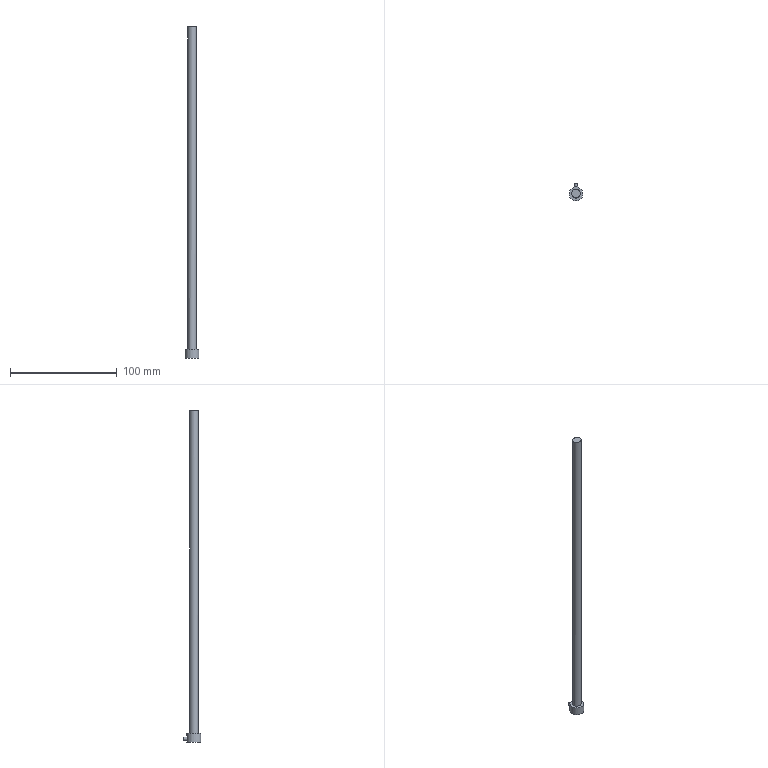Part | STEP file | E108-11-315 | 1 solid | 8 faces | box 13 x 16.5 x 310.586 mm | volume 16274 mm3 | cylinder 3 | plane 3 | spline 1 | cone 1 | commonest cylinder face diameters 3 x1 8 x1 13 x1
STEP:
#1=CARTESIAN_POINT('',(0.,0.,0.));
#2=DIRECTION('',(0.,0.,1.));
#3=DIRECTION('',(1.,0.,0.));
#4=AXIS2_PLACEMENT_3D('',#1,#2,#3);
#5=CARTESIAN_POINT('',(-3.864,1.032,309.65));
#6=VERTEX_POINT('',#5);
#7=CARTESIAN_POINT('',(-3.864,1.032,309.65));
#8=CARTESIAN_POINT('',(-3.979,0.6025,309.652));
#9=CARTESIAN_POINT('',(-4.022,0.147,309.665));
#10=CARTESIAN_POINT('',(-3.989,-0.2963,309.686));
#11=CARTESIAN_POINT('',(-3.956,-0.7395,309.708));
#12=CARTESIAN_POINT('',(-3.847,-1.183,309.739));
#13=CARTESIAN_POINT('',(-3.671,-1.589,309.777));
#14=CARTESIAN_POINT('',(-3.494,-1.998,309.816));
#15=CARTESIAN_POINT('',(-3.245,-2.381,309.862));
#16=CARTESIAN_POINT('',(-2.944,-2.708,309.911));
#17=CARTESIAN_POINT('',(-2.641,-3.038,309.961));
#18=CARTESIAN_POINT('',(-2.277,-3.319,310.016));
#19=CARTESIAN_POINT('',(-1.882,-3.53,310.071));
#20=CARTESIAN_POINT('',(-1.484,-3.742,310.126));
#21=CARTESIAN_POINT('',(-1.045,-3.887,310.183));
#22=CARTESIAN_POINT('',(-0.5993,-3.955,310.236));
#23=CARTESIAN_POINT('',(-0.1533,-4.022,310.289));
#24=CARTESIAN_POINT('',(0.3111,-4.013,310.339));
#25=CARTESIAN_POINT('',(0.7551,-3.928,310.383));
#26=CARTESIAN_POINT('',(1.197,-3.843,310.427));
#27=CARTESIAN_POINT('',(1.631,-3.68,310.466));
#28=CARTESIAN_POINT('',(2.021,-3.452,310.496));
#29=CARTESIAN_POINT('',(2.407,-3.226,310.527));
#30=CARTESIAN_POINT('',(2.761,-2.929,310.55));
#31=CARTESIAN_POINT('',(3.051,-2.586,310.565));
#32=CARTESIAN_POINT('',(3.34,-2.246,310.58));
#33=CARTESIAN_POINT('',(3.574,-1.851,310.587));
#34=CARTESIAN_POINT('',(3.734,-1.434,310.585));
#35=CARTESIAN_POINT('',(3.894,-1.018,310.584));
#36=CARTESIAN_POINT('',(3.984,-0.5693,310.575));
#37=CARTESIAN_POINT('',(3.998,-0.1245,310.559));
#38=CARTESIAN_POINT('',(4.012,0.3207,310.543));
#39=CARTESIAN_POINT('',(3.95,0.774,310.52));
#40=CARTESIAN_POINT('',(3.816,1.198,310.491));
#41=CARTESIAN_POINT('',(3.683,1.624,310.462));
#42=CARTESIAN_POINT('',(3.474,2.032,310.426));
#43=CARTESIAN_POINT('',(3.208,2.389,310.387));
#44=CARTESIAN_POINT('',(2.941,2.748,310.347));
#45=CARTESIAN_POINT('',(2.608,3.065,310.302));
#46=CARTESIAN_POINT('',(2.238,3.315,310.255));
#47=CARTESIAN_POINT('',(1.866,3.567,310.208));
#48=CARTESIAN_POINT('',(1.445,3.757,310.157));
#49=CARTESIAN_POINT('',(1.011,3.87,310.107));
#50=CARTESIAN_POINT('',(0.5759,3.984,310.056));
#51=CARTESIAN_POINT('',(0.1147,4.024,310.004));
#52=CARTESIAN_POINT('',(-0.3341,3.986,309.956));
#53=CARTESIAN_POINT('',(-0.7831,3.948,309.907));
#54=CARTESIAN_POINT('',(-1.232,3.832,309.86));
#55=CARTESIAN_POINT('',(-1.644,3.647,309.819));
#56=CARTESIAN_POINT('',(-2.054,3.462,309.778));
#57=CARTESIAN_POINT('',(-2.438,3.203,309.742));
#58=CARTESIAN_POINT('',(-2.764,2.891,309.714));
#59=CARTESIAN_POINT('',(-3.088,2.582,309.687));
#60=CARTESIAN_POINT('',(-3.363,2.212,309.667));
#61=CARTESIAN_POINT('',(-3.566,1.812,309.657));
#62=CARTESIAN_POINT('',(-3.692,1.564,309.651));
#63=CARTESIAN_POINT('',(-3.793,1.301,309.649));
#64=CARTESIAN_POINT('',(-3.864,1.032,309.65));
#65=B_SPLINE_CURVE_WITH_KNOTS('',3,(#7,#8,#9,#10,#11,#12,#13,#14,#15,#16,#17,#18,#19,#20,#21,#22,#23,#24,#25,#26,#27,#28,#29,#30,#31,#32,#33,#34,#35,#36,#37,#38,#39,#40,#41,#42,#43,#44,#45,#46,#47,#48,#49,#50,#51,#52,#53,#54,#55,#56,#57,#58,#59,#60,#61,#62,#63,#64),.UNSPECIFIED.,.T.,.F.,(1,3,3,3,3,3,3,3,3,3,3,3,3,3,3,3,3,3,3,3,3,1),(-0.03296,0.,0.0532,0.1064,0.1598,0.2137,0.2679,0.3222,0.3763,0.43,0.4834,0.5367,0.5899,0.6434,0.6971,0.751,0.8052,0.8594,0.9134,0.967,1.,1.053),.UNSPECIFIED.);
#66=CARTESIAN_POINT('',(0.,0.,108.));
#67=DIRECTION('',(0.,0.,-1.));
#68=DIRECTION('',(-1.,0.,0.));
#69=AXIS2_PLACEMENT_3D('',#66,#67,#68);
#70=CYLINDRICAL_SURFACE('',#69,4.);
#71=CARTESIAN_POINT('',(6.544,-201.65));
#72=CARTESIAN_POINT('',(6.521,-201.651));
#73=CARTESIAN_POINT('',(6.473,-201.653));
#74=CARTESIAN_POINT('',(6.401,-201.658));
#75=CARTESIAN_POINT('',(6.329,-201.666));
#76=CARTESIAN_POINT('',(6.258,-201.677));
#77=CARTESIAN_POINT('',(6.186,-201.69));
#78=CARTESIAN_POINT('',(6.115,-201.706));
#79=CARTESIAN_POINT('',(6.043,-201.725));
#80=CARTESIAN_POINT('',(5.972,-201.745));
#81=CARTESIAN_POINT('',(5.9,-201.768));
#82=CARTESIAN_POINT('',(5.829,-201.793));
#83=CARTESIAN_POINT('',(5.758,-201.82));
#84=CARTESIAN_POINT('',(5.686,-201.848));
#85=CARTESIAN_POINT('',(5.615,-201.878));
#86=CARTESIAN_POINT('',(5.544,-201.909));
#87=CARTESIAN_POINT('',(5.473,-201.941));
#88=CARTESIAN_POINT('',(5.402,-201.975));
#89=CARTESIAN_POINT('',(5.33,-202.009));
#90=CARTESIAN_POINT('',(5.259,-202.043));
#91=CARTESIAN_POINT('',(5.188,-202.078));
#92=CARTESIAN_POINT('',(5.117,-202.113));
#93=CARTESIAN_POINT('',(5.046,-202.148));
#94=CARTESIAN_POINT('',(4.975,-202.182));
#95=CARTESIAN_POINT('',(4.904,-202.217));
#96=CARTESIAN_POINT('',(4.833,-202.25));
#97=CARTESIAN_POINT('',(4.762,-202.282));
#98=CARTESIAN_POINT('',(4.69,-202.314));
#99=CARTESIAN_POINT('',(4.619,-202.344));
#100=CARTESIAN_POINT('',(4.548,-202.373));
#101=CARTESIAN_POINT('',(4.477,-202.401));
#102=CARTESIAN_POINT('',(4.405,-202.427));
#103=CARTESIAN_POINT('',(4.334,-202.451));
#104=CARTESIAN_POINT('',(4.262,-202.474));
#105=CARTESIAN_POINT('',(4.191,-202.494));
#106=CARTESIAN_POINT('',(4.12,-202.513));
#107=CARTESIAN_POINT('',(4.048,-202.53));
#108=CARTESIAN_POINT('',(3.976,-202.544));
#109=CARTESIAN_POINT('',(3.905,-202.557));
#110=CARTESIAN_POINT('',(3.834,-202.567));
#111=CARTESIAN_POINT('',(3.762,-202.575));
#112=CARTESIAN_POINT('',(3.69,-202.581));
#113=CARTESIAN_POINT('',(3.618,-202.584));
#114=CARTESIAN_POINT('',(3.547,-202.586));
#115=CARTESIAN_POINT('',(3.476,-202.585));
#116=CARTESIAN_POINT('',(3.404,-202.583));
#117=CARTESIAN_POINT('',(3.332,-202.578));
#118=CARTESIAN_POINT('',(3.26,-202.571));
#119=CARTESIAN_POINT('',(3.189,-202.562));
#120=CARTESIAN_POINT('',(3.117,-202.551));
#121=CARTESIAN_POINT('',(3.046,-202.538));
#122=CARTESIAN_POINT('',(2.974,-202.524));
#123=CARTESIAN_POINT('',(2.902,-202.508));
#124=CARTESIAN_POINT('',(2.831,-202.49));
#125=CARTESIAN_POINT('',(2.76,-202.47));
#126=CARTESIAN_POINT('',(2.688,-202.449));
#127=CARTESIAN_POINT('',(2.617,-202.426));
#128=CARTESIAN_POINT('',(2.545,-202.402));
#129=CARTESIAN_POINT('',(2.474,-202.377));
#130=CARTESIAN_POINT('',(2.403,-202.351));
#131=CARTESIAN_POINT('',(2.331,-202.323));
#132=CARTESIAN_POINT('',(2.26,-202.295));
#133=CARTESIAN_POINT('',(2.189,-202.265));
#134=CARTESIAN_POINT('',(2.118,-202.235));
#135=CARTESIAN_POINT('',(2.047,-202.205));
#136=CARTESIAN_POINT('',(1.975,-202.173));
#137=CARTESIAN_POINT('',(1.904,-202.142));
#138=CARTESIAN_POINT('',(1.833,-202.11));
#139=CARTESIAN_POINT('',(1.762,-202.078));
#140=CARTESIAN_POINT('',(1.691,-202.046));
#141=CARTESIAN_POINT('',(1.619,-202.014));
#142=CARTESIAN_POINT('',(1.548,-201.982));
#143=CARTESIAN_POINT('',(1.477,-201.951));
#144=CARTESIAN_POINT('',(1.406,-201.921));
#145=CARTESIAN_POINT('',(1.335,-201.891));
#146=CARTESIAN_POINT('',(1.263,-201.863));
#147=CARTESIAN_POINT('',(1.192,-201.835));
#148=CARTESIAN_POINT('',(1.121,-201.809));
#149=CARTESIAN_POINT('',(1.049,-201.784));
#150=CARTESIAN_POINT('',(0.9778,-201.761));
#151=CARTESIAN_POINT('',(0.9062,-201.74));
#152=CARTESIAN_POINT('',(0.8348,-201.721));
#153=CARTESIAN_POINT('',(0.7637,-201.704));
#154=CARTESIAN_POINT('',(0.6921,-201.688));
#155=CARTESIAN_POINT('',(0.6203,-201.676));
#156=CARTESIAN_POINT('',(0.5485,-201.665));
#157=CARTESIAN_POINT('',(0.4773,-201.657));
#158=CARTESIAN_POINT('',(0.4052,-201.652));
#159=CARTESIAN_POINT('',(0.3331,-201.65));
#160=CARTESIAN_POINT('',(0.285,-201.65));
#161=CARTESIAN_POINT('',(0.2611,-201.65));
#162=B_SPLINE_CURVE_WITH_KNOTS('',3,(#71,#72,#73,#74,#75,#76,#77,#78,#79,#80,#81,#82,#83,#84,#85,#86,#87,#88,#89,#90,#91,#92,#93,#94,#95,#96,#97,#98,#99,#100,#101,#102,#103,#104,#105,#106,#107,#108,#109,#110,#111,#112,#113,#114,#115,#116,#117,#118,#119,#120,#121,#122,#123,#124,#125,#126,#127,#128,#129,#130,#131,#132,#133,#134,#135,#136,#137,#138,#139,#140,#141,#142,#143,#144,#145,#146,#147,#148,#149,#150,#151,#152,#153,#154,#155,#156,#157,#158,#159,#160,#161),.UNSPECIFIED.,.F.,.F.,(4,1,1,1,1,1,1,1,1,1,1,1,1,1,1,1,1,1,1,1,1,1,1,1,1,1,1,1,1,1,1,1,1,1,1,1,1,1,1,1,1,1,1,1,1,1,1,1,1,1,1,1,1,1,1,1,1,1,1,1,1,1,1,1,1,1,1,1,1,1,1,1,1,1,1,1,1,1,1,1,1,1,1,1,1,1,1,1,4),(0.,0.01136,0.02273,0.03409,0.04545,0.05682,0.06818,0.07955,0.09091,0.1023,0.1136,0.125,0.1364,0.1477,0.1591,0.1705,0.1818,0.1932,0.2045,0.2159,0.2273,0.2386,0.25,0.2614,0.2727,0.2841,0.2955,0.3068,0.3182,0.3295,0.3409,0.3523,0.3636,0.375,0.3864,0.3977,0.4091,0.4205,0.4318,0.4432,0.4545,0.4659,0.4773,0.4886,0.5,0.5114,0.5227,0.5341,0.5455,0.5568,0.5682,0.5795,0.5909,0.6023,0.6136,0.625,0.6364,0.6477,0.6591,0.6705,0.6818,0.6932,0.7045,0.7159,0.7273,0.7386,0.75,0.7614,0.7727,0.7841,0.7955,0.8068,0.8182,0.8295,0.8409,0.8523,0.8636,0.875,0.8864,0.8977,0.9091,0.9205,0.9318,0.9432,0.9545,0.9659,0.9773,0.9886,1.),.QUASI_UNIFORM_KNOTS.);
#163=(GEOMETRIC_REPRESENTATION_CONTEXT(2)PARAMETRIC_REPRESENTATION_CONTEXT()REPRESENTATION_CONTEXT('',''));
#164=DEFINITIONAL_REPRESENTATION('',(#162),#163);
#165=PCURVE('',#70,#164);
#166=CARTESIAN_POINT('',(-9.172,-4.749,309.144));
#167=CARTESIAN_POINT('',(-3.761,-4.747,309.952));
#168=CARTESIAN_POINT('',(1.689,-4.745,310.577));
#169=CARTESIAN_POINT('',(7.189,-4.743,311.013));
#170=CARTESIAN_POINT('',(-9.178,-0.6696,308.983));
#171=CARTESIAN_POINT('',(-3.769,-0.6675,309.792));
#172=CARTESIAN_POINT('',(1.679,-0.6653,310.418));
#173=CARTESIAN_POINT('',(7.176,-0.6632,310.854));
#174=CARTESIAN_POINT('',(-9.185,3.41,308.821));
#175=CARTESIAN_POINT('',(-3.778,3.412,309.631));
#176=CARTESIAN_POINT('',(1.667,3.414,310.258));
#177=CARTESIAN_POINT('',(7.161,3.416,310.695));
#178=CARTESIAN_POINT('',(-9.194,7.49,308.658));
#179=CARTESIAN_POINT('',(-3.79,7.492,309.469));
#180=CARTESIAN_POINT('',(1.653,7.494,310.097));
#181=CARTESIAN_POINT('',(7.144,7.496,310.536));
#182=B_SPLINE_SURFACE_WITH_KNOTS('',3,3,((#166,#167,#168,#169),(#170,#171,#172,#173),(#174,#175,#176,#177),(#178,#179,#180,#181)),.UNSPECIFIED.,.F.,.F.,.F.,(4,4),(4,4),(0.,1.),(0.,1.),.PIECEWISE_BEZIER_KNOTS.);
#183=CARTESIAN_POINT('',(0.4722,0.3269));
#184=CARTESIAN_POINT('',(0.4647,0.3254));
#185=CARTESIAN_POINT('',(0.4495,0.3228));
#186=CARTESIAN_POINT('',(0.4264,0.3201));
#187=CARTESIAN_POINT('',(0.403,0.3186));
#188=CARTESIAN_POINT('',(0.3795,0.3183));
#189=CARTESIAN_POINT('',(0.3563,0.3194));
#190=CARTESIAN_POINT('',(0.3331,0.3217));
#191=CARTESIAN_POINT('',(0.3101,0.3252));
#192=CARTESIAN_POINT('',(0.2876,0.3299));
#193=CARTESIAN_POINT('',(0.2656,0.3358));
#194=CARTESIAN_POINT('',(0.2444,0.3429));
#195=CARTESIAN_POINT('',(0.2238,0.3511));
#196=CARTESIAN_POINT('',(0.204,0.3604));
#197=CARTESIAN_POINT('',(0.1852,0.3707));
#198=CARTESIAN_POINT('',(0.1674,0.382));
#199=CARTESIAN_POINT('',(0.1509,0.3941));
#200=CARTESIAN_POINT('',(0.1354,0.4072));
#201=CARTESIAN_POINT('',(0.1212,0.421));
#202=CARTESIAN_POINT('',(0.1084,0.4356));
#203=CARTESIAN_POINT('',(0.09706,0.4507));
#204=CARTESIAN_POINT('',(0.08717,0.4664));
#205=CARTESIAN_POINT('',(0.07877,0.4826));
#206=CARTESIAN_POINT('',(0.07191,0.4993));
#207=CARTESIAN_POINT('',(0.06664,0.5162));
#208=CARTESIAN_POINT('',(0.06303,0.5333));
#209=CARTESIAN_POINT('',(0.06108,0.5507));
#210=CARTESIAN_POINT('',(0.06076,0.5681));
#211=CARTESIAN_POINT('',(0.06208,0.5855));
#212=CARTESIAN_POINT('',(0.06505,0.6028));
#213=CARTESIAN_POINT('',(0.06965,0.6198));
#214=CARTESIAN_POINT('',(0.07592,0.6366));
#215=CARTESIAN_POINT('',(0.08378,0.653));
#216=CARTESIAN_POINT('',(0.09318,0.669));
#217=CARTESIAN_POINT('',(0.104,0.6845));
#218=CARTESIAN_POINT('',(0.1163,0.6992));
#219=CARTESIAN_POINT('',(0.1301,0.7134));
#220=CARTESIAN_POINT('',(0.1452,0.7268));
#221=CARTESIAN_POINT('',(0.1616,0.7393));
#222=CARTESIAN_POINT('',(0.1789,0.7509));
#223=CARTESIAN_POINT('',(0.1975,0.7616));
#224=CARTESIAN_POINT('',(0.2171,0.7713));
#225=CARTESIAN_POINT('',(0.2375,0.7799));
#226=CARTESIAN_POINT('',(0.2587,0.7874));
#227=CARTESIAN_POINT('',(0.2804,0.7938));
#228=CARTESIAN_POINT('',(0.3028,0.7989));
#229=CARTESIAN_POINT('',(0.3257,0.8029));
#230=CARTESIAN_POINT('',(0.3489,0.8056));
#231=CARTESIAN_POINT('',(0.3722,0.8072));
#232=CARTESIAN_POINT('',(0.3955,0.8074));
#233=CARTESIAN_POINT('',(0.4189,0.8064));
#234=CARTESIAN_POINT('',(0.4422,0.8042));
#235=CARTESIAN_POINT('',(0.4651,0.8007));
#236=CARTESIAN_POINT('',(0.4876,0.7961));
#237=CARTESIAN_POINT('',(0.5095,0.7902));
#238=CARTESIAN_POINT('',(0.5309,0.7832));
#239=CARTESIAN_POINT('',(0.5516,0.775));
#240=CARTESIAN_POINT('',(0.5714,0.7658));
#241=CARTESIAN_POINT('',(0.5901,0.7556));
#242=CARTESIAN_POINT('',(0.6079,0.7444));
#243=CARTESIAN_POINT('',(0.6246,0.7323));
#244=CARTESIAN_POINT('',(0.6401,0.7193));
#245=CARTESIAN_POINT('',(0.6543,0.7055));
#246=CARTESIAN_POINT('',(0.6671,0.6911));
#247=CARTESIAN_POINT('',(0.6785,0.6759));
#248=CARTESIAN_POINT('',(0.6884,0.6602));
#249=CARTESIAN_POINT('',(0.6968,0.6439));
#250=CARTESIAN_POINT('',(0.7037,0.6274));
#251=CARTESIAN_POINT('',(0.7089,0.6105));
#252=CARTESIAN_POINT('',(0.7125,0.5933));
#253=CARTESIAN_POINT('',(0.7144,0.5759));
#254=CARTESIAN_POINT('',(0.7148,0.5584));
#255=CARTESIAN_POINT('',(0.7134,0.5411));
#256=CARTESIAN_POINT('',(0.7104,0.5239));
#257=CARTESIAN_POINT('',(0.7058,0.5067));
#258=CARTESIAN_POINT('',(0.6995,0.4898));
#259=CARTESIAN_POINT('',(0.6917,0.4734));
#260=CARTESIAN_POINT('',(0.6823,0.4574));
#261=CARTESIAN_POINT('',(0.6714,0.442));
#262=CARTESIAN_POINT('',(0.6591,0.427));
#263=CARTESIAN_POINT('',(0.6453,0.4128));
#264=CARTESIAN_POINT('',(0.6303,0.3994));
#265=CARTESIAN_POINT('',(0.6141,0.3868));
#266=CARTESIAN_POINT('',(0.5966,0.3751));
#267=CARTESIAN_POINT('',(0.578,0.3644));
#268=CARTESIAN_POINT('',(0.5584,0.3546));
#269=CARTESIAN_POINT('',(0.5381,0.346));
#270=CARTESIAN_POINT('',(0.5168,0.3384));
#271=CARTESIAN_POINT('',(0.4948,0.3319));
#272=CARTESIAN_POINT('',(0.4798,0.3285));
#273=CARTESIAN_POINT('',(0.4722,0.3269));
#274=B_SPLINE_CURVE_WITH_KNOTS('',3,(#183,#184,#185,#186,#187,#188,#189,#190,#191,#192,#193,#194,#195,#196,#197,#198,#199,#200,#201,#202,#203,#204,#205,#206,#207,#208,#209,#210,#211,#212,#213,#214,#215,#216,#217,#218,#219,#220,#221,#222,#223,#224,#225,#226,#227,#228,#229,#230,#231,#232,#233,#234,#235,#236,#237,#238,#239,#240,#241,#242,#243,#244,#245,#246,#247,#248,#249,#250,#251,#252,#253,#254,#255,#256,#257,#258,#259,#260,#261,#262,#263,#264,#265,#266,#267,#268,#269,#270,#271,#272,#273),.UNSPECIFIED.,.T.,.F.,(4,1,1,1,1,1,1,1,1,1,1,1,1,1,1,1,1,1,1,1,1,1,1,1,1,1,1,1,1,1,1,1,1,1,1,1,1,1,1,1,1,1,1,1,1,1,1,1,1,1,1,1,1,1,1,1,1,1,1,1,1,1,1,1,1,1,1,1,1,1,1,1,1,1,1,1,1,1,1,1,1,1,1,1,1,1,1,1,4),(0.,0.01136,0.02273,0.03409,0.04545,0.05682,0.06818,0.07955,0.09091,0.1023,0.1136,0.125,0.1364,0.1477,0.1591,0.1705,0.1818,0.1932,0.2045,0.2159,0.2273,0.2386,0.25,0.2614,0.2727,0.2841,0.2955,0.3068,0.3182,0.3295,0.3409,0.3523,0.3636,0.375,0.3864,0.3977,0.4091,0.4205,0.4318,0.4432,0.4545,0.4659,0.4773,0.4886,0.5,0.5114,0.5227,0.5341,0.5455,0.5568,0.5682,0.5795,0.5909,0.6023,0.6136,0.625,0.6364,0.6477,0.6591,0.6705,0.6818,0.6932,0.7045,0.7159,0.7273,0.7386,0.75,0.7614,0.7727,0.7841,0.7955,0.8068,0.8182,0.8295,0.8409,0.8523,0.8636,0.875,0.8864,0.8977,0.9091,0.9205,0.9318,0.9432,0.9545,0.9659,0.9773,0.9886,1.),.QUASI_UNIFORM_KNOTS.);
#275=(GEOMETRIC_REPRESENTATION_CONTEXT(2)PARAMETRIC_REPRESENTATION_CONTEXT()REPRESENTATION_CONTEXT('',''));
#276=DEFINITIONAL_REPRESENTATION('',(#274),#275);
#277=PCURVE('',#182,#276);
#278=SURFACE_CURVE('',#65,(#165,#277),.PCURVE_S1.);
#279=EDGE_CURVE('',#6,#6,#278,.T.);
#280=ORIENTED_EDGE('',*,*,#279,.F.);
#281=CARTESIAN_POINT('',(-3.864,1.032,8.));
#282=VERTEX_POINT('',#281);
#283=CARTESIAN_POINT('',(-3.864,1.032,309.65));
#284=CARTESIAN_POINT('',(-3.864,1.032,8.));
#285=B_SPLINE_CURVE_WITH_KNOTS('',1,(#283,#284),.UNSPECIFIED.,.F.,.F.,(2,2),(-201.65,100.),.PIECEWISE_BEZIER_KNOTS.);
#286=CARTESIAN_POINT('',(6.544,0.));
#287=DIRECTION('',(0.,1.));
#288=VECTOR('',#287,1.);
#289=LINE('',#286,#288);
#290=(GEOMETRIC_REPRESENTATION_CONTEXT(2)PARAMETRIC_REPRESENTATION_CONTEXT()REPRESENTATION_CONTEXT('',''));
#291=DEFINITIONAL_REPRESENTATION('',(#289),#290);
#292=PCURVE('',#70,#291);
#293=CARTESIAN_POINT('',(0.2611,0.));
#294=DIRECTION('',(0.,1.));
#295=VECTOR('',#294,1.);
#296=LINE('',#293,#295);
#297=(GEOMETRIC_REPRESENTATION_CONTEXT(2)PARAMETRIC_REPRESENTATION_CONTEXT()REPRESENTATION_CONTEXT('',''));
#298=DEFINITIONAL_REPRESENTATION('',(#296),#297);
#299=PCURVE('',#70,#298);
#300=SEAM_CURVE('',#285,(#292,#299),.PCURVE_S1.);
#301=EDGE_CURVE('',#6,#282,#300,.T.);
#302=ORIENTED_EDGE('',*,*,#301,.T.);
#303=CARTESIAN_POINT('',(4.,0.,8.));
#304=VERTEX_POINT('',#303);
#305=CARTESIAN_POINT('',(0.,0.,8.));
#306=DIRECTION('',(0.,0.,1.));
#307=DIRECTION('',(1.,0.,0.));
#308=AXIS2_PLACEMENT_3D('',#305,#306,#307);
#309=CIRCLE('',#308,4.);
#310=CARTESIAN_POINT('',(9.425,100.));
#311=DIRECTION('',(-1.,0.));
#312=VECTOR('',#311,1.);
#313=LINE('',#310,#312);
#314=(GEOMETRIC_REPRESENTATION_CONTEXT(2)PARAMETRIC_REPRESENTATION_CONTEXT()REPRESENTATION_CONTEXT('',''));
#315=DEFINITIONAL_REPRESENTATION('',(#313),#314);
#316=PCURVE('',#70,#315);
#317=CARTESIAN_POINT('',(0.,0.,8.));
#318=DIRECTION('',(0.,0.,-1.));
#319=DIRECTION('',(1.,0.,0.));
#320=AXIS2_PLACEMENT_3D('',#317,#318,#319);
#321=PLANE('',#320);
#322=CARTESIAN_POINT('',(4.,0.));
#323=CARTESIAN_POINT('',(4.,-6.928));
#324=CARTESIAN_POINT('',(-2.,-3.464));
#325=CARTESIAN_POINT('',(-8.,0.));
#326=CARTESIAN_POINT('',(-2.,3.464));
#327=CARTESIAN_POINT('',(4.,6.928));
#328=CARTESIAN_POINT('',(4.,0.));
#329=(BOUNDED_CURVE()B_SPLINE_CURVE(2,(#322,#323,#324,#325,#326,#327,#328),.UNSPECIFIED.,.T.,.F.)B_SPLINE_CURVE_WITH_KNOTS((1,2,2,2,2,1),(-2.094,0.,2.094,4.189,6.283,8.378),.UNSPECIFIED.)CURVE()GEOMETRIC_REPRESENTATION_ITEM()RATIONAL_B_SPLINE_CURVE((1.,0.5,1.,0.5,1.,0.5,1.))REPRESENTATION_ITEM(''));
#330=(GEOMETRIC_REPRESENTATION_CONTEXT(2)PARAMETRIC_REPRESENTATION_CONTEXT()REPRESENTATION_CONTEXT('',''));
#331=DEFINITIONAL_REPRESENTATION('',(#329),#330);
#332=PCURVE('',#321,#331);
#333=SURFACE_CURVE('',#309,(#316,#332),.PCURVE_S1.);
#334=EDGE_CURVE('',#282,#304,#333,.T.);
#335=ORIENTED_EDGE('',*,*,#334,.T.);
#336=CARTESIAN_POINT('',(0.,0.,8.));
#337=DIRECTION('',(0.,0.,1.));
#338=DIRECTION('',(1.,0.,0.));
#339=AXIS2_PLACEMENT_3D('',#336,#337,#338);
#340=CIRCLE('',#339,4.);
#341=CARTESIAN_POINT('',(3.142,100.));
#342=DIRECTION('',(-1.,0.));
#343=VECTOR('',#342,1.);
#344=LINE('',#341,#343);
#345=(GEOMETRIC_REPRESENTATION_CONTEXT(2)PARAMETRIC_REPRESENTATION_CONTEXT()REPRESENTATION_CONTEXT('',''));
#346=DEFINITIONAL_REPRESENTATION('',(#344),#345);
#347=PCURVE('',#70,#346);
#348=CARTESIAN_POINT('',(4.,0.));
#349=CARTESIAN_POINT('',(4.,-6.928));
#350=CARTESIAN_POINT('',(-2.,-3.464));
#351=CARTESIAN_POINT('',(-8.,0.));
#352=CARTESIAN_POINT('',(-2.,3.464));
#353=CARTESIAN_POINT('',(4.,6.928));
#354=CARTESIAN_POINT('',(4.,0.));
#355=(BOUNDED_CURVE()B_SPLINE_CURVE(2,(#348,#349,#350,#351,#352,#353,#354),.UNSPECIFIED.,.T.,.F.)B_SPLINE_CURVE_WITH_KNOTS((1,2,2,2,2,1),(-2.094,0.,2.094,4.189,6.283,8.378),.UNSPECIFIED.)CURVE()GEOMETRIC_REPRESENTATION_ITEM()RATIONAL_B_SPLINE_CURVE((1.,0.5,1.,0.5,1.,0.5,1.))REPRESENTATION_ITEM(''));
#356=(GEOMETRIC_REPRESENTATION_CONTEXT(2)PARAMETRIC_REPRESENTATION_CONTEXT()REPRESENTATION_CONTEXT('',''));
#357=DEFINITIONAL_REPRESENTATION('',(#355),#356);
#358=PCURVE('',#321,#357);
#359=SURFACE_CURVE('',#340,(#347,#358),.PCURVE_S1.);
#360=EDGE_CURVE('',#304,#282,#359,.T.);
#361=ORIENTED_EDGE('',*,*,#360,.T.);
#362=ORIENTED_EDGE('',*,*,#301,.F.);
#363=EDGE_LOOP('',(#280,#302,#335,#361,#362));
#364=FACE_BOUND('',#363,.T.);
#365=ADVANCED_FACE('',(#364),#70,.T.);
#366=ORIENTED_EDGE('',*,*,#279,.F.);
#367=EDGE_LOOP('',(#366));
#368=FACE_BOUND('',#367,.F.);
#369=ADVANCED_FACE('',(#368),#182,.F.);
#370=CARTESIAN_POINT('',(6.5,0.,0.));
#371=VERTEX_POINT('',#370);
#372=CARTESIAN_POINT('',(-6.5,0.,0.));
#373=VERTEX_POINT('',#372);
#374=CARTESIAN_POINT('',(0.,0.,0.));
#375=DIRECTION('',(0.,0.,-1.));
#376=DIRECTION('',(-1.,0.,0.));
#377=AXIS2_PLACEMENT_3D('',#374,#375,#376);
#378=CIRCLE('',#377,6.5);
#379=CARTESIAN_POINT('',(0.,0.,8.));
#380=DIRECTION('',(0.,0.,-1.));
#381=DIRECTION('',(1.,0.,0.));
#382=AXIS2_PLACEMENT_3D('',#379,#380,#381);
#383=CYLINDRICAL_SURFACE('',#382,6.5);
#384=CARTESIAN_POINT('',(-3.142,8.));
#385=DIRECTION('',(1.,0.));
#386=VECTOR('',#385,1.);
#387=LINE('',#384,#386);
#388=(GEOMETRIC_REPRESENTATION_CONTEXT(2)PARAMETRIC_REPRESENTATION_CONTEXT()REPRESENTATION_CONTEXT('',''));
#389=DEFINITIONAL_REPRESENTATION('',(#387),#388);
#390=PCURVE('',#383,#389);
#391=CARTESIAN_POINT('',(240.,-1000.,0.));
#392=DIRECTION('',(0.,0.,1.));
#393=DIRECTION('',(-1.,0.,0.));
#394=AXIS2_PLACEMENT_3D('',#391,#392,#393);
#395=PLANE('',#394);
#396=CARTESIAN_POINT('',(246.5,-1000.));
#397=CARTESIAN_POINT('',(246.5,-1011.258));
#398=CARTESIAN_POINT('',(236.75,-1005.629));
#399=CARTESIAN_POINT('',(227.,-1000.));
#400=CARTESIAN_POINT('',(236.75,-994.371));
#401=CARTESIAN_POINT('',(246.5,-988.742));
#402=CARTESIAN_POINT('',(246.5,-1000.));
#403=(BOUNDED_CURVE()B_SPLINE_CURVE(2,(#396,#397,#398,#399,#400,#401,#402),.UNSPECIFIED.,.T.,.F.)B_SPLINE_CURVE_WITH_KNOTS((1,2,2,2,2,1),(-2.094,0.,2.094,4.189,6.283,8.378),.UNSPECIFIED.)CURVE()GEOMETRIC_REPRESENTATION_ITEM()RATIONAL_B_SPLINE_CURVE((1.,0.5,1.,0.5,1.,0.5,1.))REPRESENTATION_ITEM(''));
#404=(GEOMETRIC_REPRESENTATION_CONTEXT(2)PARAMETRIC_REPRESENTATION_CONTEXT()REPRESENTATION_CONTEXT('',''));
#405=DEFINITIONAL_REPRESENTATION('',(#403),#404);
#406=PCURVE('',#395,#405);
#407=SURFACE_CURVE('',#378,(#390,#406),.PCURVE_S1.);
#408=EDGE_CURVE('',#371,#373,#407,.T.);
#409=ORIENTED_EDGE('',*,*,#408,.F.);
#410=CARTESIAN_POINT('',(6.5,0.,8.));
#411=VERTEX_POINT('',#410);
#412=CARTESIAN_POINT('',(6.5,0.,8.));
#413=CARTESIAN_POINT('',(6.5,0.,0.));
#414=B_SPLINE_CURVE_WITH_KNOTS('',1,(#412,#413),.UNSPECIFIED.,.F.,.F.,(2,2),(0.,8.),.PIECEWISE_BEZIER_KNOTS.);
#415=CARTESIAN_POINT('',(0.,0.));
#416=DIRECTION('',(0.,1.));
#417=VECTOR('',#416,1.);
#418=LINE('',#415,#417);
#419=(GEOMETRIC_REPRESENTATION_CONTEXT(2)PARAMETRIC_REPRESENTATION_CONTEXT()REPRESENTATION_CONTEXT('',''));
#420=DEFINITIONAL_REPRESENTATION('',(#418),#419);
#421=PCURVE('',#383,#420);
#422=CARTESIAN_POINT('',(6.283,0.));
#423=DIRECTION('',(0.,1.));
#424=VECTOR('',#423,1.);
#425=LINE('',#422,#424);
#426=(GEOMETRIC_REPRESENTATION_CONTEXT(2)PARAMETRIC_REPRESENTATION_CONTEXT()REPRESENTATION_CONTEXT('',''));
#427=DEFINITIONAL_REPRESENTATION('',(#425),#426);
#428=PCURVE('',#383,#427);
#429=SEAM_CURVE('',#414,(#421,#428),.PCURVE_S1.);
#430=EDGE_CURVE('',#411,#371,#429,.T.);
#431=ORIENTED_EDGE('',*,*,#430,.F.);
#432=CARTESIAN_POINT('',(0.,0.,8.));
#433=DIRECTION('',(0.,0.,-1.));
#434=DIRECTION('',(1.,0.,0.));
#435=AXIS2_PLACEMENT_3D('',#432,#433,#434);
#436=CIRCLE('',#435,6.5);
#437=CARTESIAN_POINT('',(0.,0.));
#438=DIRECTION('',(1.,0.));
#439=VECTOR('',#438,1.);
#440=LINE('',#437,#439);
#441=(GEOMETRIC_REPRESENTATION_CONTEXT(2)PARAMETRIC_REPRESENTATION_CONTEXT()REPRESENTATION_CONTEXT('',''));
#442=DEFINITIONAL_REPRESENTATION('',(#440),#441);
#443=PCURVE('',#383,#442);
#444=CARTESIAN_POINT('',(0.,0.));
#445=DIRECTION('',(1.,0.));
#446=AXIS2_PLACEMENT_2D('',#444,#445);
#447=CIRCLE('',#446,6.5);
#448=(GEOMETRIC_REPRESENTATION_CONTEXT(2)PARAMETRIC_REPRESENTATION_CONTEXT()REPRESENTATION_CONTEXT('',''));
#449=DEFINITIONAL_REPRESENTATION('',(#447),#448);
#450=PCURVE('',#321,#449);
#451=SURFACE_CURVE('',#436,(#443,#450),.PCURVE_S1.);
#452=EDGE_CURVE('',#411,#411,#451,.T.);
#453=ORIENTED_EDGE('',*,*,#452,.T.);
#454=ORIENTED_EDGE('',*,*,#430,.T.);
#455=CARTESIAN_POINT('',(0.,0.,0.));
#456=DIRECTION('',(0.,0.,-1.));
#457=DIRECTION('',(-1.,0.,0.));
#458=AXIS2_PLACEMENT_3D('',#455,#456,#457);
#459=CIRCLE('',#458,6.5);
#460=CARTESIAN_POINT('',(3.142,8.));
#461=DIRECTION('',(1.,0.));
#462=VECTOR('',#461,1.);
#463=LINE('',#460,#462);
#464=(GEOMETRIC_REPRESENTATION_CONTEXT(2)PARAMETRIC_REPRESENTATION_CONTEXT()REPRESENTATION_CONTEXT('',''));
#465=DEFINITIONAL_REPRESENTATION('',(#463),#464);
#466=PCURVE('',#383,#465);
#467=CARTESIAN_POINT('',(246.5,-1000.));
#468=CARTESIAN_POINT('',(246.5,-1011.258));
#469=CARTESIAN_POINT('',(236.75,-1005.629));
#470=CARTESIAN_POINT('',(227.,-1000.));
#471=CARTESIAN_POINT('',(236.75,-994.371));
#472=CARTESIAN_POINT('',(246.5,-988.742));
#473=CARTESIAN_POINT('',(246.5,-1000.));
#474=(BOUNDED_CURVE()B_SPLINE_CURVE(2,(#467,#468,#469,#470,#471,#472,#473),.UNSPECIFIED.,.T.,.F.)B_SPLINE_CURVE_WITH_KNOTS((1,2,2,2,2,1),(-2.094,0.,2.094,4.189,6.283,8.378),.UNSPECIFIED.)CURVE()GEOMETRIC_REPRESENTATION_ITEM()RATIONAL_B_SPLINE_CURVE((1.,0.5,1.,0.5,1.,0.5,1.))REPRESENTATION_ITEM(''));
#475=(GEOMETRIC_REPRESENTATION_CONTEXT(2)PARAMETRIC_REPRESENTATION_CONTEXT()REPRESENTATION_CONTEXT('',''));
#476=DEFINITIONAL_REPRESENTATION('',(#474),#475);
#477=PCURVE('',#395,#476);
#478=SURFACE_CURVE('',#459,(#466,#477),.PCURVE_S1.);
#479=EDGE_CURVE('',#373,#371,#478,.T.);
#480=ORIENTED_EDGE('',*,*,#479,.F.);
#481=EDGE_LOOP('',(#409,#431,#453,#454,#480));
#482=FACE_BOUND('',#481,.T.);
#483=CARTESIAN_POINT('',(0.,6.5,1.5));
#484=VERTEX_POINT('',#483);
#485=CARTESIAN_POINT('',(0.,6.5,1.5));
#486=CARTESIAN_POINT('',(0.1654,6.5,1.5));
#487=CARTESIAN_POINT('',(0.3332,6.493,1.528));
#488=CARTESIAN_POINT('',(0.4892,6.482,1.582));
#489=CARTESIAN_POINT('',(0.6451,6.47,1.636));
#490=CARTESIAN_POINT('',(0.7936,6.453,1.717));
#491=CARTESIAN_POINT('',(0.9231,6.434,1.818));
#492=CARTESIAN_POINT('',(1.055,6.415,1.92));
#493=CARTESIAN_POINT('',(1.17,6.394,2.047));
#494=CARTESIAN_POINT('',(1.261,6.377,2.187));
#495=CARTESIAN_POINT('',(1.352,6.358,2.329));
#496=CARTESIAN_POINT('',(1.421,6.343,2.49));
#497=CARTESIAN_POINT('',(1.46,6.334,2.655));
#498=CARTESIAN_POINT('',(1.498,6.325,2.817));
#499=CARTESIAN_POINT('',(1.509,6.322,2.989));
#500=CARTESIAN_POINT('',(1.492,6.326,3.155));
#501=CARTESIAN_POINT('',(1.475,6.33,3.318));
#502=CARTESIAN_POINT('',(1.431,6.341,3.48));
#503=CARTESIAN_POINT('',(1.362,6.356,3.628));
#504=CARTESIAN_POINT('',(1.293,6.37,3.777));
#505=CARTESIAN_POINT('',(1.199,6.39,3.917));
#506=CARTESIAN_POINT('',(1.085,6.409,4.035));
#507=CARTESIAN_POINT('',(0.9695,6.428,4.157));
#508=CARTESIAN_POINT('',(0.8309,6.448,4.26));
#509=CARTESIAN_POINT('',(0.6809,6.464,4.337));
#510=CARTESIAN_POINT('',(0.5305,6.48,4.413));
#511=CARTESIAN_POINT('',(0.3642,6.492,4.465));
#512=CARTESIAN_POINT('',(0.1962,6.497,4.487));
#513=CARTESIAN_POINT('',(0.03191,6.502,4.509));
#514=CARTESIAN_POINT('',(-0.1386,6.501,4.503));
#515=CARTESIAN_POINT('',(-0.3008,6.493,4.47));
#516=CARTESIAN_POINT('',(-0.4611,6.486,4.437));
#517=CARTESIAN_POINT('',(-0.6177,6.472,4.377));
#518=CARTESIAN_POINT('',(-0.7583,6.456,4.294));
#519=CARTESIAN_POINT('',(-0.9011,6.439,4.211));
#520=CARTESIAN_POINT('',(-1.031,6.419,4.102));
#521=CARTESIAN_POINT('',(-1.139,6.399,3.976));
#522=CARTESIAN_POINT('',(-1.249,6.38,3.848));
#523=CARTESIAN_POINT('',(-1.338,6.361,3.699));
#524=CARTESIAN_POINT('',(-1.399,6.348,3.541));
#525=CARTESIAN_POINT('',(-1.46,6.334,3.384));
#526=CARTESIAN_POINT('',(-1.494,6.326,3.214));
#527=CARTESIAN_POINT('',(-1.499,6.325,3.046));
#528=CARTESIAN_POINT('',(-1.504,6.324,2.881));
#529=CARTESIAN_POINT('',(-1.482,6.329,2.714));
#530=CARTESIAN_POINT('',(-1.433,6.34,2.557));
#531=CARTESIAN_POINT('',(-1.385,6.351,2.4));
#532=CARTESIAN_POINT('',(-1.309,6.367,2.25));
#533=CARTESIAN_POINT('',(-1.214,6.386,2.119));
#534=CARTESIAN_POINT('',(-1.116,6.404,1.984));
#535=CARTESIAN_POINT('',(-0.9937,6.425,1.864));
#536=CARTESIAN_POINT('',(-0.8569,6.443,1.769));
#537=CARTESIAN_POINT('',(-0.7182,6.462,1.672));
#538=CARTESIAN_POINT('',(-0.5604,6.478,1.598));
#539=CARTESIAN_POINT('',(-0.3967,6.488,1.553));
#540=CARTESIAN_POINT('',(-0.2682,6.496,1.518));
#541=CARTESIAN_POINT('',(-0.1335,6.5,1.5));
#542=CARTESIAN_POINT('',(0.,6.5,1.5));
#543=B_SPLINE_CURVE_WITH_KNOTS('',3,(#485,#486,#487,#488,#489,#490,#491,#492,#493,#494,#495,#496,#497,#498,#499,#500,#501,#502,#503,#504,#505,#506,#507,#508,#509,#510,#511,#512,#513,#514,#515,#516,#517,#518,#519,#520,#521,#522,#523,#524,#525,#526,#527,#528,#529,#530,#531,#532,#533,#534,#535,#536,#537,#538,#539,#540,#541,#542),.UNSPECIFIED.,.T.,.F.,(1,3,3,3,3,3,3,3,3,3,3,3,3,3,3,3,3,3,3,3,3,1),(-0.04234,0.,0.05275,0.1054,0.159,0.2132,0.2665,0.3187,0.3713,0.4252,0.4793,0.5321,0.5843,0.6373,0.6915,0.7453,0.7978,0.85,0.9034,0.9577,1.,1.053),.UNSPECIFIED.);
#544=CARTESIAN_POINT('',(4.712,6.5));
#545=CARTESIAN_POINT('',(4.718,6.5));
#546=CARTESIAN_POINT('',(4.729,6.497));
#547=CARTESIAN_POINT('',(4.745,6.486));
#548=CARTESIAN_POINT('',(4.762,6.467));
#549=CARTESIAN_POINT('',(4.778,6.44));
#550=CARTESIAN_POINT('',(4.793,6.406));
#551=CARTESIAN_POINT('',(4.809,6.365));
#552=CARTESIAN_POINT('',(4.823,6.317));
#553=CARTESIAN_POINT('',(4.838,6.262));
#554=CARTESIAN_POINT('',(4.851,6.201));
#555=CARTESIAN_POINT('',(4.864,6.135));
#556=CARTESIAN_POINT('',(4.876,6.062));
#557=CARTESIAN_POINT('',(4.888,5.983));
#558=CARTESIAN_POINT('',(4.898,5.9));
#559=CARTESIAN_POINT('',(4.908,5.813));
#560=CARTESIAN_POINT('',(4.916,5.721));
#561=CARTESIAN_POINT('',(4.924,5.625));
#562=CARTESIAN_POINT('',(4.93,5.526));
#563=CARTESIAN_POINT('',(4.936,5.424));
#564=CARTESIAN_POINT('',(4.94,5.321));
#565=CARTESIAN_POINT('',(4.943,5.215));
#566=CARTESIAN_POINT('',(4.945,5.108));
#567=CARTESIAN_POINT('',(4.945,5.));
#568=CARTESIAN_POINT('',(4.945,4.893));
#569=CARTESIAN_POINT('',(4.943,4.787));
#570=CARTESIAN_POINT('',(4.94,4.681));
#571=CARTESIAN_POINT('',(4.936,4.576));
#572=CARTESIAN_POINT('',(4.93,4.474));
#573=CARTESIAN_POINT('',(4.924,4.376));
#574=CARTESIAN_POINT('',(4.916,4.28));
#575=CARTESIAN_POINT('',(4.908,4.188));
#576=CARTESIAN_POINT('',(4.898,4.1));
#577=CARTESIAN_POINT('',(4.888,4.017));
#578=CARTESIAN_POINT('',(4.877,3.939));
#579=CARTESIAN_POINT('',(4.864,3.866));
#580=CARTESIAN_POINT('',(4.851,3.799));
#581=CARTESIAN_POINT('',(4.838,3.738));
#582=CARTESIAN_POINT('',(4.824,3.683));
#583=CARTESIAN_POINT('',(4.809,3.635));
#584=CARTESIAN_POINT('',(4.793,3.594));
#585=CARTESIAN_POINT('',(4.778,3.56));
#586=CARTESIAN_POINT('',(4.762,3.533));
#587=CARTESIAN_POINT('',(4.745,3.514));
#588=CARTESIAN_POINT('',(4.729,3.503));
#589=CARTESIAN_POINT('',(4.713,3.499));
#590=CARTESIAN_POINT('',(4.696,3.503));
#591=CARTESIAN_POINT('',(4.679,3.514));
#592=CARTESIAN_POINT('',(4.663,3.533));
#593=CARTESIAN_POINT('',(4.647,3.56));
#594=CARTESIAN_POINT('',(4.632,3.594));
#595=CARTESIAN_POINT('',(4.616,3.635));
#596=CARTESIAN_POINT('',(4.601,3.683));
#597=CARTESIAN_POINT('',(4.587,3.737));
#598=CARTESIAN_POINT('',(4.574,3.798));
#599=CARTESIAN_POINT('',(4.561,3.865));
#600=CARTESIAN_POINT('',(4.548,3.938));
#601=CARTESIAN_POINT('',(4.537,4.016));
#602=CARTESIAN_POINT('',(4.527,4.099));
#603=CARTESIAN_POINT('',(4.517,4.187));
#604=CARTESIAN_POINT('',(4.508,4.279));
#605=CARTESIAN_POINT('',(4.501,4.375));
#606=CARTESIAN_POINT('',(4.494,4.473));
#607=CARTESIAN_POINT('',(4.489,4.575));
#608=CARTESIAN_POINT('',(4.485,4.679));
#609=CARTESIAN_POINT('',(4.482,4.785));
#610=CARTESIAN_POINT('',(4.48,4.892));
#611=CARTESIAN_POINT('',(4.479,4.999));
#612=CARTESIAN_POINT('',(4.48,5.106));
#613=CARTESIAN_POINT('',(4.482,5.213));
#614=CARTESIAN_POINT('',(4.485,5.319));
#615=CARTESIAN_POINT('',(4.489,5.423));
#616=CARTESIAN_POINT('',(4.494,5.524));
#617=CARTESIAN_POINT('',(4.501,5.624));
#618=CARTESIAN_POINT('',(4.508,5.72));
#619=CARTESIAN_POINT('',(4.517,5.812));
#620=CARTESIAN_POINT('',(4.526,5.899));
#621=CARTESIAN_POINT('',(4.537,5.982));
#622=CARTESIAN_POINT('',(4.548,6.061));
#623=CARTESIAN_POINT('',(4.56,6.134));
#624=CARTESIAN_POINT('',(4.573,6.201));
#625=CARTESIAN_POINT('',(4.587,6.262));
#626=CARTESIAN_POINT('',(4.601,6.316));
#627=CARTESIAN_POINT('',(4.616,6.364));
#628=CARTESIAN_POINT('',(4.631,6.406));
#629=CARTESIAN_POINT('',(4.647,6.44));
#630=CARTESIAN_POINT('',(4.663,6.466));
#631=CARTESIAN_POINT('',(4.679,6.486));
#632=CARTESIAN_POINT('',(4.696,6.497));
#633=CARTESIAN_POINT('',(4.707,6.5));
#634=CARTESIAN_POINT('',(4.712,6.5));
#635=B_SPLINE_CURVE_WITH_KNOTS('',3,(#544,#545,#546,#547,#548,#549,#550,#551,#552,#553,#554,#555,#556,#557,#558,#559,#560,#561,#562,#563,#564,#565,#566,#567,#568,#569,#570,#571,#572,#573,#574,#575,#576,#577,#578,#579,#580,#581,#582,#583,#584,#585,#586,#587,#588,#589,#590,#591,#592,#593,#594,#595,#596,#597,#598,#599,#600,#601,#602,#603,#604,#605,#606,#607,#608,#609,#610,#611,#612,#613,#614,#615,#616,#617,#618,#619,#620,#621,#622,#623,#624,#625,#626,#627,#628,#629,#630,#631,#632,#633,#634),.UNSPECIFIED.,.T.,.F.,(4,1,1,1,1,1,1,1,1,1,1,1,1,1,1,1,1,1,1,1,1,1,1,1,1,1,1,1,1,1,1,1,1,1,1,1,1,1,1,1,1,1,1,1,1,1,1,1,1,1,1,1,1,1,1,1,1,1,1,1,1,1,1,1,1,1,1,1,1,1,1,1,1,1,1,1,1,1,1,1,1,1,1,1,1,1,1,1,4),(0.,0.01136,0.02273,0.03409,0.04545,0.05682,0.06818,0.07955,0.09091,0.1023,0.1136,0.125,0.1364,0.1477,0.1591,0.1705,0.1818,0.1932,0.2045,0.2159,0.2273,0.2386,0.25,0.2614,0.2727,0.2841,0.2955,0.3068,0.3182,0.3295,0.3409,0.3523,0.3636,0.375,0.3864,0.3977,0.4091,0.4205,0.4318,0.4432,0.4545,0.4659,0.4773,0.4886,0.5,0.5114,0.5227,0.5341,0.5455,0.5568,0.5682,0.5795,0.5909,0.6023,0.6136,0.625,0.6364,0.6477,0.6591,0.6705,0.6818,0.6932,0.7045,0.7159,0.7273,0.7386,0.75,0.7614,0.7727,0.7841,0.7955,0.8068,0.8182,0.8295,0.8409,0.8523,0.8636,0.875,0.8864,0.8977,0.9091,0.9205,0.9318,0.9432,0.9545,0.9659,0.9773,0.9886,1.),.QUASI_UNIFORM_KNOTS.);
#636=(GEOMETRIC_REPRESENTATION_CONTEXT(2)PARAMETRIC_REPRESENTATION_CONTEXT()REPRESENTATION_CONTEXT('',''));
#637=DEFINITIONAL_REPRESENTATION('',(#635),#636);
#638=PCURVE('',#383,#637);
#639=CARTESIAN_POINT('',(0.,2.,3.));
#640=DIRECTION('',(0.,1.,0.));
#641=DIRECTION('',(0.,0.,-1.));
#642=AXIS2_PLACEMENT_3D('',#639,#640,#641);
#643=CYLINDRICAL_SURFACE('',#642,1.5);
#644=CARTESIAN_POINT('',(6.283,4.5));
#645=CARTESIAN_POINT('',(6.259,4.5));
#646=CARTESIAN_POINT('',(6.212,4.499));
#647=CARTESIAN_POINT('',(6.14,4.497));
#648=CARTESIAN_POINT('',(6.068,4.492));
#649=CARTESIAN_POINT('',(5.997,4.486));
#650=CARTESIAN_POINT('',(5.926,4.479));
#651=CARTESIAN_POINT('',(5.854,4.47));
#652=CARTESIAN_POINT('',(5.783,4.46));
#653=CARTESIAN_POINT('',(5.711,4.449));
#654=CARTESIAN_POINT('',(5.64,4.438));
#655=CARTESIAN_POINT('',(5.569,4.425));
#656=CARTESIAN_POINT('',(5.498,4.413));
#657=CARTESIAN_POINT('',(5.427,4.4));
#658=CARTESIAN_POINT('',(5.355,4.388));
#659=CARTESIAN_POINT('',(5.284,4.376));
#660=CARTESIAN_POINT('',(5.213,4.365));
#661=CARTESIAN_POINT('',(5.142,4.355));
#662=CARTESIAN_POINT('',(5.07,4.346));
#663=CARTESIAN_POINT('',(4.999,4.338));
#664=CARTESIAN_POINT('',(4.928,4.332));
#665=CARTESIAN_POINT('',(4.856,4.328));
#666=CARTESIAN_POINT('',(4.784,4.325));
#667=CARTESIAN_POINT('',(4.713,4.324));
#668=CARTESIAN_POINT('',(4.641,4.325));
#669=CARTESIAN_POINT('',(4.57,4.328));
#670=CARTESIAN_POINT('',(4.498,4.332));
#671=CARTESIAN_POINT('',(4.426,4.339));
#672=CARTESIAN_POINT('',(4.355,4.346));
#673=CARTESIAN_POINT('',(4.283,4.355));
#674=CARTESIAN_POINT('',(4.212,4.365));
#675=CARTESIAN_POINT('',(4.141,4.376));
#676=CARTESIAN_POINT('',(4.07,4.388));
#677=CARTESIAN_POINT('',(3.998,4.4));
#678=CARTESIAN_POINT('',(3.927,4.413));
#679=CARTESIAN_POINT('',(3.856,4.425));
#680=CARTESIAN_POINT('',(3.785,4.437));
#681=CARTESIAN_POINT('',(3.714,4.449));
#682=CARTESIAN_POINT('',(3.642,4.46));
#683=CARTESIAN_POINT('',(3.571,4.47));
#684=CARTESIAN_POINT('',(3.5,4.479));
#685=CARTESIAN_POINT('',(3.428,4.486));
#686=CARTESIAN_POINT('',(3.357,4.492));
#687=CARTESIAN_POINT('',(3.285,4.497));
#688=CARTESIAN_POINT('',(3.214,4.499));
#689=CARTESIAN_POINT('',(3.142,4.5));
#690=CARTESIAN_POINT('',(3.07,4.499));
#691=CARTESIAN_POINT('',(2.999,4.497));
#692=CARTESIAN_POINT('',(2.927,4.492));
#693=CARTESIAN_POINT('',(2.856,4.486));
#694=CARTESIAN_POINT('',(2.784,4.479));
#695=CARTESIAN_POINT('',(2.713,4.47));
#696=CARTESIAN_POINT('',(2.641,4.46));
#697=CARTESIAN_POINT('',(2.57,4.449));
#698=CARTESIAN_POINT('',(2.499,4.438));
#699=CARTESIAN_POINT('',(2.428,4.425));
#700=CARTESIAN_POINT('',(2.357,4.413));
#701=CARTESIAN_POINT('',(2.285,4.4));
#702=CARTESIAN_POINT('',(2.215,4.388));
#703=CARTESIAN_POINT('',(2.143,4.376));
#704=CARTESIAN_POINT('',(2.072,4.365));
#705=CARTESIAN_POINT('',(2.,4.355));
#706=CARTESIAN_POINT('',(1.929,4.346));
#707=CARTESIAN_POINT('',(1.858,4.339));
#708=CARTESIAN_POINT('',(1.786,4.332));
#709=CARTESIAN_POINT('',(1.715,4.328));
#710=CARTESIAN_POINT('',(1.643,4.325));
#711=CARTESIAN_POINT('',(1.572,4.324));
#712=CARTESIAN_POINT('',(1.5,4.325));
#713=CARTESIAN_POINT('',(1.428,4.328));
#714=CARTESIAN_POINT('',(1.357,4.332));
#715=CARTESIAN_POINT('',(1.285,4.338));
#716=CARTESIAN_POINT('',(1.214,4.346));
#717=CARTESIAN_POINT('',(1.142,4.355));
#718=CARTESIAN_POINT('',(1.071,4.365));
#719=CARTESIAN_POINT('',(0.9995,4.376));
#720=CARTESIAN_POINT('',(0.9286,4.388));
#721=CARTESIAN_POINT('',(0.8575,4.4));
#722=CARTESIAN_POINT('',(0.7862,4.413));
#723=CARTESIAN_POINT('',(0.7149,4.425));
#724=CARTESIAN_POINT('',(0.6436,4.437));
#725=CARTESIAN_POINT('',(0.5728,4.449));
#726=CARTESIAN_POINT('',(0.5015,4.46));
#727=CARTESIAN_POINT('',(0.43,4.47));
#728=CARTESIAN_POINT('',(0.3585,4.479));
#729=CARTESIAN_POINT('',(0.2872,4.486));
#730=CARTESIAN_POINT('',(0.2157,4.492));
#731=CARTESIAN_POINT('',(0.1438,4.497));
#732=CARTESIAN_POINT('',(0.07178,4.499));
#733=CARTESIAN_POINT('',(0.02388,4.5));
#734=CARTESIAN_POINT('',(0.,4.5));
#735=B_SPLINE_CURVE_WITH_KNOTS('',3,(#644,#645,#646,#647,#648,#649,#650,#651,#652,#653,#654,#655,#656,#657,#658,#659,#660,#661,#662,#663,#664,#665,#666,#667,#668,#669,#670,#671,#672,#673,#674,#675,#676,#677,#678,#679,#680,#681,#682,#683,#684,#685,#686,#687,#688,#689,#690,#691,#692,#693,#694,#695,#696,#697,#698,#699,#700,#701,#702,#703,#704,#705,#706,#707,#708,#709,#710,#711,#712,#713,#714,#715,#716,#717,#718,#719,#720,#721,#722,#723,#724,#725,#726,#727,#728,#729,#730,#731,#732,#733,#734),.UNSPECIFIED.,.F.,.F.,(4,1,1,1,1,1,1,1,1,1,1,1,1,1,1,1,1,1,1,1,1,1,1,1,1,1,1,1,1,1,1,1,1,1,1,1,1,1,1,1,1,1,1,1,1,1,1,1,1,1,1,1,1,1,1,1,1,1,1,1,1,1,1,1,1,1,1,1,1,1,1,1,1,1,1,1,1,1,1,1,1,1,1,1,1,1,1,1,4),(0.,0.01136,0.02273,0.03409,0.04545,0.05682,0.06818,0.07955,0.09091,0.1023,0.1136,0.125,0.1364,0.1477,0.1591,0.1705,0.1818,0.1932,0.2045,0.2159,0.2273,0.2386,0.25,0.2614,0.2727,0.2841,0.2955,0.3068,0.3182,0.3295,0.3409,0.3523,0.3636,0.375,0.3864,0.3977,0.4091,0.4205,0.4318,0.4432,0.4545,0.4659,0.4773,0.4886,0.5,0.5114,0.5227,0.5341,0.5455,0.5568,0.5682,0.5795,0.5909,0.6023,0.6136,0.625,0.6364,0.6477,0.6591,0.6705,0.6818,0.6932,0.7045,0.7159,0.7273,0.7386,0.75,0.7614,0.7727,0.7841,0.7955,0.8068,0.8182,0.8295,0.8409,0.8523,0.8636,0.875,0.8864,0.8977,0.9091,0.9205,0.9318,0.9432,0.9545,0.9659,0.9773,0.9886,1.),.QUASI_UNIFORM_KNOTS.);
#736=(GEOMETRIC_REPRESENTATION_CONTEXT(2)PARAMETRIC_REPRESENTATION_CONTEXT()REPRESENTATION_CONTEXT('',''));
#737=DEFINITIONAL_REPRESENTATION('',(#735),#736);
#738=PCURVE('',#643,#737);
#739=SURFACE_CURVE('',#543,(#638,#738),.PCURVE_S1.);
#740=EDGE_CURVE('',#484,#484,#739,.T.);
#741=ORIENTED_EDGE('',*,*,#740,.T.);
#742=EDGE_LOOP('',(#741));
#743=FACE_BOUND('',#742,.T.);
#744=ADVANCED_FACE('',(#482,#743),#383,.T.);
#745=ORIENTED_EDGE('',*,*,#360,.F.);
#746=ORIENTED_EDGE('',*,*,#334,.F.);
#747=EDGE_LOOP('',(#745,#746));
#748=FACE_BOUND('',#747,.T.);
#749=ORIENTED_EDGE('',*,*,#452,.F.);
#750=EDGE_LOOP('',(#749));
#751=FACE_BOUND('',#750,.T.);
#752=ADVANCED_FACE('',(#748,#751),#321,.F.);
#753=ORIENTED_EDGE('',*,*,#479,.T.);
#754=ORIENTED_EDGE('',*,*,#408,.T.);
#755=EDGE_LOOP('',(#753,#754));
#756=FACE_BOUND('',#755,.T.);
#757=ADVANCED_FACE('',(#756),#395,.F.);
#758=CARTESIAN_POINT('',(0.,10.,1.75));
#759=VERTEX_POINT('',#758);
#760=CARTESIAN_POINT('',(0.,10.,3.));
#761=DIRECTION('',(0.,1.,0.));
#762=DIRECTION('',(0.,0.,-1.));
#763=AXIS2_PLACEMENT_3D('',#760,#761,#762);
#764=CIRCLE('',#763,1.25);
#765=CARTESIAN_POINT('',(0.,10.,3.));
#766=DIRECTION('',(0.,1.,0.));
#767=DIRECTION('',(0.,0.,-1.));
#768=AXIS2_PLACEMENT_3D('',#765,#766,#767);
#769=PLANE('',#768);
#770=CARTESIAN_POINT('',(0.,0.));
#771=DIRECTION('',(1.,0.));
#772=AXIS2_PLACEMENT_2D('',#770,#771);
#773=CIRCLE('',#772,1.25);
#774=(GEOMETRIC_REPRESENTATION_CONTEXT(2)PARAMETRIC_REPRESENTATION_CONTEXT()REPRESENTATION_CONTEXT('',''));
#775=DEFINITIONAL_REPRESENTATION('',(#773),#774);
#776=PCURVE('',#769,#775);
#777=CARTESIAN_POINT('',(0.,9.75,3.));
#778=DIRECTION('',(0.,-1.,0.));
#779=DIRECTION('',(0.,0.,1.));
#780=AXIS2_PLACEMENT_3D('',#777,#778,#779);
#781=CONICAL_SURFACE('',#780,1.5,0.7854);
#782=CARTESIAN_POINT('',(9.425,-0.25));
#783=DIRECTION('',(-1.,0.));
#784=VECTOR('',#783,1.);
#785=LINE('',#782,#784);
#786=(GEOMETRIC_REPRESENTATION_CONTEXT(2)PARAMETRIC_REPRESENTATION_CONTEXT()REPRESENTATION_CONTEXT('',''));
#787=DEFINITIONAL_REPRESENTATION('',(#785),#786);
#788=PCURVE('',#781,#787);
#789=SURFACE_CURVE('',#764,(#776,#788),.PCURVE_S1.);
#790=EDGE_CURVE('',#759,#759,#789,.T.);
#791=ORIENTED_EDGE('',*,*,#790,.T.);
#792=EDGE_LOOP('',(#791));
#793=FACE_BOUND('',#792,.T.);
#794=ADVANCED_FACE('',(#793),#769,.T.);
#795=ORIENTED_EDGE('',*,*,#790,.F.);
#796=CARTESIAN_POINT('',(0.,9.75,1.5));
#797=VERTEX_POINT('',#796);
#798=CARTESIAN_POINT('',(0.,10.,1.75));
#799=CARTESIAN_POINT('',(0.,9.75,1.5));
#800=B_SPLINE_CURVE_WITH_KNOTS('',1,(#798,#799),.UNSPECIFIED.,.F.,.F.,(2,2),(-0.3536,0.),.PIECEWISE_BEZIER_KNOTS.);
#801=CARTESIAN_POINT('',(9.425,0.));
#802=DIRECTION('',(0.,1.));
#803=VECTOR('',#802,1.);
#804=LINE('',#801,#803);
#805=(GEOMETRIC_REPRESENTATION_CONTEXT(2)PARAMETRIC_REPRESENTATION_CONTEXT()REPRESENTATION_CONTEXT('',''));
#806=DEFINITIONAL_REPRESENTATION('',(#804),#805);
#807=PCURVE('',#781,#806);
#808=CARTESIAN_POINT('',(3.142,0.));
#809=DIRECTION('',(0.,1.));
#810=VECTOR('',#809,1.);
#811=LINE('',#808,#810);
#812=(GEOMETRIC_REPRESENTATION_CONTEXT(2)PARAMETRIC_REPRESENTATION_CONTEXT()REPRESENTATION_CONTEXT('',''));
#813=DEFINITIONAL_REPRESENTATION('',(#811),#812);
#814=PCURVE('',#781,#813);
#815=SEAM_CURVE('',#800,(#807,#814),.PCURVE_S1.);
#816=EDGE_CURVE('',#759,#797,#815,.T.);
#817=ORIENTED_EDGE('',*,*,#816,.T.);
#818=CARTESIAN_POINT('',(0.,9.75,3.));
#819=DIRECTION('',(0.,-1.,0.));
#820=DIRECTION('',(0.,0.,-1.));
#821=AXIS2_PLACEMENT_3D('',#818,#819,#820);
#822=CIRCLE('',#821,1.5);
#823=CARTESIAN_POINT('',(3.142,0.));
#824=DIRECTION('',(1.,0.));
#825=VECTOR('',#824,1.);
#826=LINE('',#823,#825);
#827=(GEOMETRIC_REPRESENTATION_CONTEXT(2)PARAMETRIC_REPRESENTATION_CONTEXT()REPRESENTATION_CONTEXT('',''));
#828=DEFINITIONAL_REPRESENTATION('',(#826),#827);
#829=PCURVE('',#781,#828);
#830=CARTESIAN_POINT('',(6.283,7.75));
#831=DIRECTION('',(-1.,0.));
#832=VECTOR('',#831,1.);
#833=LINE('',#830,#832);
#834=(GEOMETRIC_REPRESENTATION_CONTEXT(2)PARAMETRIC_REPRESENTATION_CONTEXT()REPRESENTATION_CONTEXT('',''));
#835=DEFINITIONAL_REPRESENTATION('',(#833),#834);
#836=PCURVE('',#643,#835);
#837=SURFACE_CURVE('',#822,(#829,#836),.PCURVE_S1.);
#838=EDGE_CURVE('',#797,#797,#837,.T.);
#839=ORIENTED_EDGE('',*,*,#838,.F.);
#840=ORIENTED_EDGE('',*,*,#816,.F.);
#841=EDGE_LOOP('',(#795,#817,#839,#840));
#842=FACE_BOUND('',#841,.T.);
#843=ADVANCED_FACE('',(#842),#781,.T.);
#844=ORIENTED_EDGE('',*,*,#740,.F.);
#845=CARTESIAN_POINT('',(0.,6.5,1.5));
#846=CARTESIAN_POINT('',(0.,9.75,1.5));
#847=B_SPLINE_CURVE_WITH_KNOTS('',1,(#845,#846),.UNSPECIFIED.,.F.,.F.,(2,2),(4.5,7.75),.PIECEWISE_BEZIER_KNOTS.);
#848=CARTESIAN_POINT('',(6.283,0.));
#849=DIRECTION('',(0.,1.));
#850=VECTOR('',#849,1.);
#851=LINE('',#848,#850);
#852=(GEOMETRIC_REPRESENTATION_CONTEXT(2)PARAMETRIC_REPRESENTATION_CONTEXT()REPRESENTATION_CONTEXT('',''));
#853=DEFINITIONAL_REPRESENTATION('',(#851),#852);
#854=PCURVE('',#643,#853);
#855=CARTESIAN_POINT('',(0.,0.));
#856=DIRECTION('',(0.,1.));
#857=VECTOR('',#856,1.);
#858=LINE('',#855,#857);
#859=(GEOMETRIC_REPRESENTATION_CONTEXT(2)PARAMETRIC_REPRESENTATION_CONTEXT()REPRESENTATION_CONTEXT('',''));
#860=DEFINITIONAL_REPRESENTATION('',(#858),#859);
#861=PCURVE('',#643,#860);
#862=SEAM_CURVE('',#847,(#854,#861),.PCURVE_S1.);
#863=EDGE_CURVE('',#484,#797,#862,.T.);
#864=ORIENTED_EDGE('',*,*,#863,.T.);
#865=ORIENTED_EDGE('',*,*,#838,.T.);
#866=ORIENTED_EDGE('',*,*,#863,.F.);
#867=EDGE_LOOP('',(#844,#864,#865,#866));
#868=FACE_BOUND('',#867,.T.);
#869=ADVANCED_FACE('',(#868),#643,.T.);
#870=CLOSED_SHELL('',(#365,#369,#744,#752,#757,#794,#843,#869));
#871=MANIFOLD_SOLID_BREP('',#870);
#872=(LENGTH_UNIT()NAMED_UNIT(*)SI_UNIT(.MILLI.,.METRE.));
#873=UNCERTAINTY_MEASURE_WITH_UNIT(LENGTH_MEASURE(0.00005),#872,'','');
#874=(NAMED_UNIT(*)PLANE_ANGLE_UNIT()SI_UNIT($,.RADIAN.));
#875=(NAMED_UNIT(*)SI_UNIT($,.STERADIAN.)SOLID_ANGLE_UNIT());
#876=(GEOMETRIC_REPRESENTATION_CONTEXT(3)GLOBAL_UNCERTAINTY_ASSIGNED_CONTEXT((#873))GLOBAL_UNIT_ASSIGNED_CONTEXT((#872,#874,#875))REPRESENTATION_CONTEXT('',''));
#877=ADVANCED_BREP_SHAPE_REPRESENTATION('',(#4,#871),#876);